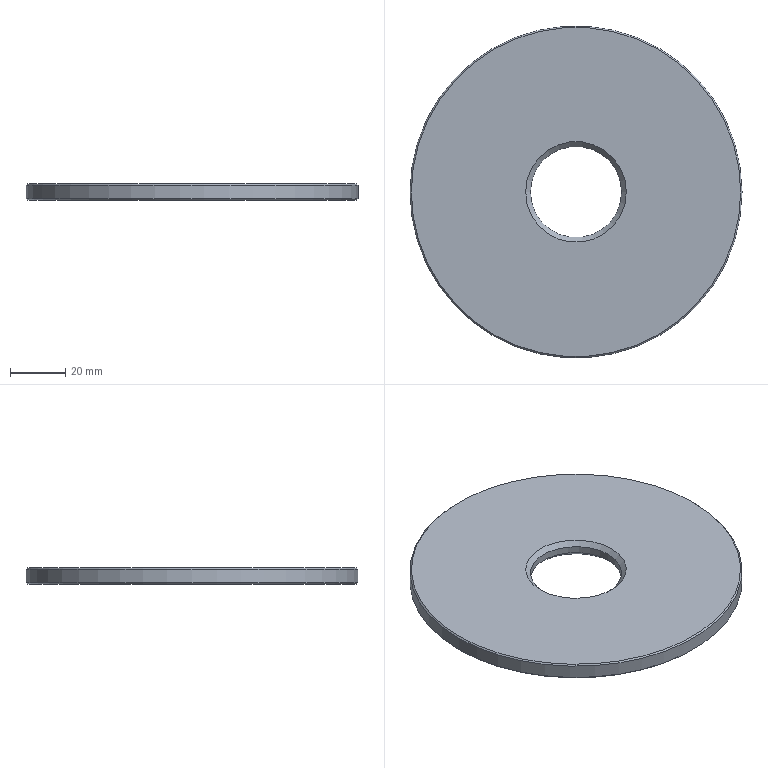Part | NX | features CHAMFER 1, CYLINDER 1, DATUM_CSYS 1, HOLE PACKAGE 1, SIMPLE HOLE 1 | 1 solid | 8 faces | box 120 x 120 x 6 mm | volume 62323 mm3 | cone 4 | plane 2 | cylinder 2 | commonest cylinder face diameters 33 x1 120 x1
STEP:
#1=CARTESIAN_POINT('',(59.5,0.,6.));
#2=VERTEX_POINT('',#1);
#3=CARTESIAN_POINT('',(0.,0.,6.));
#4=DIRECTION('',(0.,0.,1.));
#5=DIRECTION('',(1.,0.,0.));
#6=AXIS2_PLACEMENT_3D('',#3,#4,#5);
#7=CIRCLE('',#6,59.5);
#8=EDGE_CURVE('',#2,#2,#7,.T.);
#9=ORIENTED_EDGE('',*,*,#8,.T.);
#10=EDGE_LOOP('',(#9));
#11=FACE_BOUND('',#10,.T.);
#12=CARTESIAN_POINT('',(18.2,0.,6.));
#13=VERTEX_POINT('',#12);
#14=CARTESIAN_POINT('',(0.,0.,6.));
#15=DIRECTION('',(0.,0.,1.));
#16=DIRECTION('',(1.,0.,0.));
#17=AXIS2_PLACEMENT_3D('',#14,#15,#16);
#18=CIRCLE('',#17,18.2);
#19=EDGE_CURVE('',#13,#13,#18,.F.);
#20=ORIENTED_EDGE('',*,*,#19,.T.);
#21=EDGE_LOOP('',(#20));
#22=FACE_BOUND('',#21,.T.);
#23=CARTESIAN_POINT('',(0.,0.,6.));
#24=DIRECTION('',(0.,0.,1.));
#25=DIRECTION('',(1.,0.,0.));
#26=AXIS2_PLACEMENT_3D('',#23,#24,#25);
#27=PLANE('',#26);
#28=ADVANCED_FACE('',(#11,#22),#27,.T.);
#29=CARTESIAN_POINT('',(-59.5,0.,0.));
#30=VERTEX_POINT('',#29);
#31=CARTESIAN_POINT('',(0.,0.,0.));
#32=DIRECTION('',(0.,0.,-1.));
#33=DIRECTION('',(-1.,0.,0.));
#34=AXIS2_PLACEMENT_3D('',#31,#32,#33);
#35=CIRCLE('',#34,59.5);
#36=EDGE_CURVE('',#30,#30,#35,.T.);
#37=ORIENTED_EDGE('',*,*,#36,.T.);
#38=EDGE_LOOP('',(#37));
#39=FACE_BOUND('',#38,.T.);
#40=CARTESIAN_POINT('',(-18.2,0.,0.));
#41=VERTEX_POINT('',#40);
#42=CARTESIAN_POINT('',(0.,0.,0.));
#43=DIRECTION('',(0.,0.,-1.));
#44=DIRECTION('',(-1.,0.,0.));
#45=AXIS2_PLACEMENT_3D('',#42,#43,#44);
#46=CIRCLE('',#45,18.2);
#47=EDGE_CURVE('',#41,#41,#46,.F.);
#48=ORIENTED_EDGE('',*,*,#47,.T.);
#49=EDGE_LOOP('',(#48));
#50=FACE_BOUND('',#49,.T.);
#51=CARTESIAN_POINT('',(0.,0.,0.));
#52=DIRECTION('',(0.,0.,-1.));
#53=DIRECTION('',(-1.,0.,0.));
#54=AXIS2_PLACEMENT_3D('',#51,#52,#53);
#55=PLANE('',#54);
#56=ADVANCED_FACE('',(#39,#50),#55,.T.);
#57=CARTESIAN_POINT('',(-60.,0.,0.5));
#58=VERTEX_POINT('',#57);
#59=CARTESIAN_POINT('',(0.,0.,0.5));
#60=DIRECTION('',(0.,0.,-1.));
#61=DIRECTION('',(-1.,0.,0.));
#62=AXIS2_PLACEMENT_3D('',#59,#60,#61);
#63=CIRCLE('',#62,60.);
#64=EDGE_CURVE('',#58,#58,#63,.F.);
#65=ORIENTED_EDGE('',*,*,#64,.T.);
#66=EDGE_LOOP('',(#65));
#67=FACE_BOUND('',#66,.T.);
#68=CARTESIAN_POINT('',(60.,0.,5.5));
#69=VERTEX_POINT('',#68);
#70=CARTESIAN_POINT('',(0.,0.,5.5));
#71=DIRECTION('',(0.,0.,1.));
#72=DIRECTION('',(1.,0.,0.));
#73=AXIS2_PLACEMENT_3D('',#70,#71,#72);
#74=CIRCLE('',#73,60.);
#75=EDGE_CURVE('',#69,#69,#74,.F.);
#76=ORIENTED_EDGE('',*,*,#75,.T.);
#77=EDGE_LOOP('',(#76));
#78=FACE_BOUND('',#77,.T.);
#79=CARTESIAN_POINT('',(0.,0.,0.));
#80=DIRECTION('',(0.,0.,1.));
#81=DIRECTION('',(1.,0.,0.));
#82=AXIS2_PLACEMENT_3D('',#79,#80,#81);
#83=CYLINDRICAL_SURFACE('',#82,60.);
#84=ADVANCED_FACE('',(#67,#78),#83,.T.);
#85=CARTESIAN_POINT('',(-16.5,0.,1.7));
#86=VERTEX_POINT('',#85);
#87=CARTESIAN_POINT('',(0.,0.,1.7));
#88=DIRECTION('',(0.,0.,-1.));
#89=DIRECTION('',(-1.,0.,0.));
#90=AXIS2_PLACEMENT_3D('',#87,#88,#89);
#91=CIRCLE('',#90,16.5);
#92=EDGE_CURVE('',#86,#86,#91,.T.);
#93=ORIENTED_EDGE('',*,*,#92,.T.);
#94=EDGE_LOOP('',(#93));
#95=FACE_BOUND('',#94,.T.);
#96=CARTESIAN_POINT('',(16.5,0.,4.3));
#97=VERTEX_POINT('',#96);
#98=CARTESIAN_POINT('',(0.,0.,4.3));
#99=DIRECTION('',(0.,0.,1.));
#100=DIRECTION('',(1.,0.,0.));
#101=AXIS2_PLACEMENT_3D('',#98,#99,#100);
#102=CIRCLE('',#101,16.5);
#103=EDGE_CURVE('',#97,#97,#102,.T.);
#104=ORIENTED_EDGE('',*,*,#103,.T.);
#105=EDGE_LOOP('',(#104));
#106=FACE_BOUND('',#105,.T.);
#107=CARTESIAN_POINT('',(0.,0.,6.));
#108=DIRECTION('',(0.,0.,-1.));
#109=DIRECTION('',(-1.,0.,0.));
#110=AXIS2_PLACEMENT_3D('',#107,#108,#109);
#111=CYLINDRICAL_SURFACE('',#110,16.5);
#112=ADVANCED_FACE('',(#95,#106),#111,.F.);
#113=ORIENTED_EDGE('',*,*,#103,.F.);
#114=EDGE_LOOP('',(#113));
#115=FACE_BOUND('',#114,.T.);
#116=ORIENTED_EDGE('',*,*,#19,.F.);
#117=EDGE_LOOP('',(#116));
#118=FACE_BOUND('',#117,.T.);
#119=CARTESIAN_POINT('',(0.,0.,6.));
#120=DIRECTION('',(0.,0.,1.));
#121=DIRECTION('',(1.,0.,0.));
#122=AXIS2_PLACEMENT_3D('',#119,#120,#121);
#123=CONICAL_SURFACE('',#122,18.2,0.7854);
#124=ADVANCED_FACE('',(#115,#118),#123,.F.);
#125=ORIENTED_EDGE('',*,*,#47,.F.);
#126=EDGE_LOOP('',(#125));
#127=FACE_BOUND('',#126,.T.);
#128=ORIENTED_EDGE('',*,*,#92,.F.);
#129=EDGE_LOOP('',(#128));
#130=FACE_BOUND('',#129,.T.);
#131=CARTESIAN_POINT('',(0.,0.,1.7));
#132=DIRECTION('',(0.,0.,-1.));
#133=DIRECTION('',(-1.,0.,0.));
#134=AXIS2_PLACEMENT_3D('',#131,#132,#133);
#135=CONICAL_SURFACE('',#134,16.5,0.7854);
#136=ADVANCED_FACE('',(#127,#130),#135,.F.);
#137=ORIENTED_EDGE('',*,*,#36,.F.);
#138=EDGE_LOOP('',(#137));
#139=FACE_BOUND('',#138,.T.);
#140=ORIENTED_EDGE('',*,*,#64,.F.);
#141=EDGE_LOOP('',(#140));
#142=FACE_BOUND('',#141,.T.);
#143=CARTESIAN_POINT('',(0.,0.,0.5));
#144=DIRECTION('',(0.,0.,1.));
#145=DIRECTION('',(1.,0.,0.));
#146=AXIS2_PLACEMENT_3D('',#143,#144,#145);
#147=CONICAL_SURFACE('',#146,60.,0.7854);
#148=ADVANCED_FACE('',(#139,#142),#147,.T.);
#149=ORIENTED_EDGE('',*,*,#8,.F.);
#150=EDGE_LOOP('',(#149));
#151=FACE_BOUND('',#150,.T.);
#152=ORIENTED_EDGE('',*,*,#75,.F.);
#153=EDGE_LOOP('',(#152));
#154=FACE_BOUND('',#153,.T.);
#155=CARTESIAN_POINT('',(0.,0.,5.5));
#156=DIRECTION('',(0.,0.,-1.));
#157=DIRECTION('',(-1.,0.,0.));
#158=AXIS2_PLACEMENT_3D('',#155,#156,#157);
#159=CONICAL_SURFACE('',#158,60.,0.7854);
#160=ADVANCED_FACE('',(#151,#154),#159,.T.);
#161=CLOSED_SHELL('',(#28,#56,#84,#112,#124,#136,#148,#160));
#162=MANIFOLD_SOLID_BREP('',#161);
#163=(LENGTH_UNIT()NAMED_UNIT(*)SI_UNIT(.MILLI.,.METRE.));
#164=UNCERTAINTY_MEASURE_WITH_UNIT(LENGTH_MEASURE(0.00001),#163,'','');
#165=(NAMED_UNIT(*)PLANE_ANGLE_UNIT()SI_UNIT($,.RADIAN.));
#166=(NAMED_UNIT(*)SI_UNIT($,.STERADIAN.)SOLID_ANGLE_UNIT());
#167=(GEOMETRIC_REPRESENTATION_CONTEXT(3)GLOBAL_UNCERTAINTY_ASSIGNED_CONTEXT((#164))GLOBAL_UNIT_ASSIGNED_CONTEXT((#163,#165,#166))REPRESENTATION_CONTEXT('',''));
#168=ADVANCED_BREP_SHAPE_REPRESENTATION('',(#162),#167);